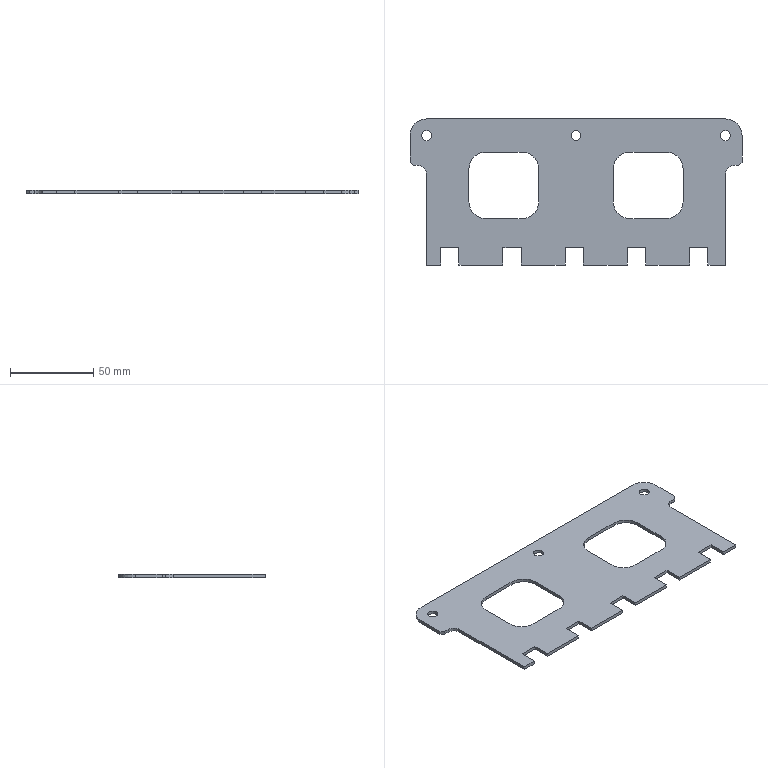Part | STEP file | GLSJ-10-18_default | 1 solid | 58 faces | box 200 x 88 x 2 mm | volume 25026 mm3 | plane 40 | cylinder 18 | commonest cylinder face diameters 20 x10 6 x6 10 x2